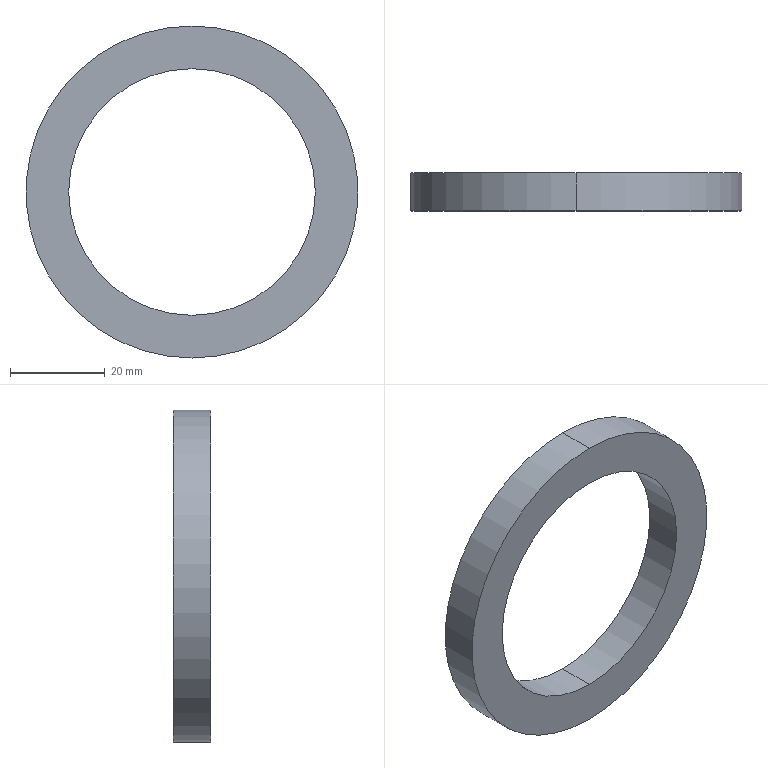Part | SolidWorks | features Extrusion 1 | 1 solid | 6 faces | box 70 x 8 x 70 mm | volume 13798 mm3 | cylinder 4 | plane 2 | commonest cylinder face diameters 52 x2 70 x2
STEP:
#1=CARTESIAN_POINT('',(0.,8.,-26.));
#2=VERTEX_POINT('',#1);
#3=CARTESIAN_POINT('',(0.,8.,26.));
#4=VERTEX_POINT('',#3);
#5=CARTESIAN_POINT('',(0.,8.,0.));
#6=DIRECTION('',(0.,1.,0.));
#7=DIRECTION('',(0.,0.,1.));
#8=AXIS2_PLACEMENT_3D('',#5,#6,#7);
#9=CIRCLE('',#8,26.);
#10=EDGE_CURVE('',#2,#4,#9,.T.);
#11=ORIENTED_EDGE('',*,*,#10,.T.);
#12=CARTESIAN_POINT('',(0.,0.,26.));
#13=VERTEX_POINT('',#12);
#14=CARTESIAN_POINT('',(0.,8.,26.));
#15=DIRECTION('',(0.,-1.,0.));
#16=VECTOR('',#15,1000.);
#17=LINE('',#14,#16);
#18=EDGE_CURVE('',#4,#13,#17,.T.);
#19=ORIENTED_EDGE('',*,*,#18,.T.);
#20=CARTESIAN_POINT('',(0.,0.,-26.));
#21=VERTEX_POINT('',#20);
#22=CARTESIAN_POINT('',(0.,0.,0.));
#23=DIRECTION('',(0.,1.,0.));
#24=DIRECTION('',(0.,0.,1.));
#25=AXIS2_PLACEMENT_3D('',#22,#23,#24);
#26=CIRCLE('',#25,26.);
#27=EDGE_CURVE('',#21,#13,#26,.T.);
#28=ORIENTED_EDGE('',*,*,#27,.F.);
#29=CARTESIAN_POINT('',(0.,8.,-26.));
#30=DIRECTION('',(0.,-1.,0.));
#31=VECTOR('',#30,1000.);
#32=LINE('',#29,#31);
#33=EDGE_CURVE('',#2,#21,#32,.T.);
#34=ORIENTED_EDGE('',*,*,#33,.F.);
#35=EDGE_LOOP('',(#11,#19,#28,#34));
#36=FACE_OUTER_BOUND('',#35,.T.);
#37=CARTESIAN_POINT('',(0.,8.,0.));
#38=DIRECTION('',(0.,-1.,0.));
#39=DIRECTION('',(0.,0.,-1.));
#40=AXIS2_PLACEMENT_3D('',#37,#38,#39);
#41=CYLINDRICAL_SURFACE('',#40,26.);
#42=ADVANCED_FACE('',(#36),#41,.F.);
#43=CARTESIAN_POINT('',(0.,8.,35.));
#44=VERTEX_POINT('',#43);
#45=CARTESIAN_POINT('',(0.,8.,-35.));
#46=VERTEX_POINT('',#45);
#47=CARTESIAN_POINT('',(0.,8.,0.));
#48=DIRECTION('',(0.,1.,0.));
#49=DIRECTION('',(0.,0.,1.));
#50=AXIS2_PLACEMENT_3D('',#47,#48,#49);
#51=CIRCLE('',#50,35.);
#52=EDGE_CURVE('',#44,#46,#51,.T.);
#53=ORIENTED_EDGE('',*,*,#52,.F.);
#54=CARTESIAN_POINT('',(0.,0.,35.));
#55=VERTEX_POINT('',#54);
#56=CARTESIAN_POINT('',(0.,8.,35.));
#57=DIRECTION('',(0.,-1.,0.));
#58=VECTOR('',#57,1000.);
#59=LINE('',#56,#58);
#60=EDGE_CURVE('',#44,#55,#59,.T.);
#61=ORIENTED_EDGE('',*,*,#60,.T.);
#62=CARTESIAN_POINT('',(0.,0.,-35.));
#63=VERTEX_POINT('',#62);
#64=CARTESIAN_POINT('',(0.,0.,0.));
#65=DIRECTION('',(0.,1.,0.));
#66=DIRECTION('',(0.,0.,1.));
#67=AXIS2_PLACEMENT_3D('',#64,#65,#66);
#68=CIRCLE('',#67,35.);
#69=EDGE_CURVE('',#55,#63,#68,.T.);
#70=ORIENTED_EDGE('',*,*,#69,.T.);
#71=CARTESIAN_POINT('',(0.,8.,-35.));
#72=DIRECTION('',(0.,-1.,0.));
#73=VECTOR('',#72,1000.);
#74=LINE('',#71,#73);
#75=EDGE_CURVE('',#46,#63,#74,.T.);
#76=ORIENTED_EDGE('',*,*,#75,.F.);
#77=EDGE_LOOP('',(#53,#61,#70,#76));
#78=FACE_OUTER_BOUND('',#77,.T.);
#79=CARTESIAN_POINT('',(0.,8.,0.));
#80=DIRECTION('',(0.,-1.,0.));
#81=DIRECTION('',(0.,0.,-1.));
#82=AXIS2_PLACEMENT_3D('',#79,#80,#81);
#83=CYLINDRICAL_SURFACE('',#82,35.);
#84=ADVANCED_FACE('',(#78),#83,.T.);
#85=CARTESIAN_POINT('',(0.,8.,0.));
#86=DIRECTION('',(0.,1.,0.));
#87=DIRECTION('',(0.,0.,1.));
#88=AXIS2_PLACEMENT_3D('',#85,#86,#87);
#89=CIRCLE('',#88,35.);
#90=EDGE_CURVE('',#46,#44,#89,.T.);
#91=ORIENTED_EDGE('',*,*,#90,.T.);
#92=ORIENTED_EDGE('',*,*,#52,.T.);
#93=EDGE_LOOP('',(#91,#92));
#94=FACE_OUTER_BOUND('',#93,.T.);
#95=ORIENTED_EDGE('',*,*,#10,.F.);
#96=CARTESIAN_POINT('',(0.,8.,0.));
#97=DIRECTION('',(0.,1.,0.));
#98=DIRECTION('',(0.,0.,1.));
#99=AXIS2_PLACEMENT_3D('',#96,#97,#98);
#100=CIRCLE('',#99,26.);
#101=EDGE_CURVE('',#4,#2,#100,.T.);
#102=ORIENTED_EDGE('',*,*,#101,.F.);
#103=EDGE_LOOP('',(#95,#102));
#104=FACE_BOUND('',#103,.T.);
#105=CARTESIAN_POINT('',(0.,8.,0.));
#106=DIRECTION('',(0.,1.,0.));
#107=DIRECTION('',(0.,0.,1.));
#108=AXIS2_PLACEMENT_3D('',#105,#106,#107);
#109=PLANE('',#108);
#110=ADVANCED_FACE('',(#94,#104),#109,.T.);
#111=CARTESIAN_POINT('',(0.,0.,0.));
#112=DIRECTION('',(0.,1.,0.));
#113=DIRECTION('',(0.,0.,1.));
#114=AXIS2_PLACEMENT_3D('',#111,#112,#113);
#115=CIRCLE('',#114,35.);
#116=EDGE_CURVE('',#63,#55,#115,.T.);
#117=ORIENTED_EDGE('',*,*,#116,.F.);
#118=ORIENTED_EDGE('',*,*,#69,.F.);
#119=EDGE_LOOP('',(#117,#118));
#120=FACE_OUTER_BOUND('',#119,.T.);
#121=ORIENTED_EDGE('',*,*,#27,.T.);
#122=CARTESIAN_POINT('',(0.,0.,0.));
#123=DIRECTION('',(0.,1.,0.));
#124=DIRECTION('',(0.,0.,1.));
#125=AXIS2_PLACEMENT_3D('',#122,#123,#124);
#126=CIRCLE('',#125,26.);
#127=EDGE_CURVE('',#13,#21,#126,.T.);
#128=ORIENTED_EDGE('',*,*,#127,.T.);
#129=EDGE_LOOP('',(#121,#128));
#130=FACE_BOUND('',#129,.T.);
#131=CARTESIAN_POINT('',(0.,0.,0.));
#132=DIRECTION('',(0.,1.,0.));
#133=DIRECTION('',(0.,0.,1.));
#134=AXIS2_PLACEMENT_3D('',#131,#132,#133);
#135=PLANE('',#134);
#136=ADVANCED_FACE('',(#120,#130),#135,.F.);
#137=ORIENTED_EDGE('',*,*,#60,.F.);
#138=ORIENTED_EDGE('',*,*,#90,.F.);
#139=ORIENTED_EDGE('',*,*,#75,.T.);
#140=ORIENTED_EDGE('',*,*,#116,.T.);
#141=EDGE_LOOP('',(#137,#138,#139,#140));
#142=FACE_OUTER_BOUND('',#141,.T.);
#143=CARTESIAN_POINT('',(0.,8.,0.));
#144=DIRECTION('',(0.,-1.,0.));
#145=DIRECTION('',(0.,0.,-1.));
#146=AXIS2_PLACEMENT_3D('',#143,#144,#145);
#147=CYLINDRICAL_SURFACE('',#146,35.);
#148=ADVANCED_FACE('',(#142),#147,.T.);
#149=ORIENTED_EDGE('',*,*,#18,.F.);
#150=ORIENTED_EDGE('',*,*,#101,.T.);
#151=ORIENTED_EDGE('',*,*,#33,.T.);
#152=ORIENTED_EDGE('',*,*,#127,.F.);
#153=EDGE_LOOP('',(#149,#150,#151,#152));
#154=FACE_OUTER_BOUND('',#153,.T.);
#155=CARTESIAN_POINT('',(0.,8.,0.));
#156=DIRECTION('',(0.,-1.,0.));
#157=DIRECTION('',(0.,0.,-1.));
#158=AXIS2_PLACEMENT_3D('',#155,#156,#157);
#159=CYLINDRICAL_SURFACE('',#158,26.);
#160=ADVANCED_FACE('',(#154),#159,.F.);
#161=CLOSED_SHELL('',(#42,#84,#110,#136,#148,#160));
#162=MANIFOLD_SOLID_BREP('',#161);
#163=CARTESIAN_POINT('',(0.,0.,0.));
#164=DIRECTION('',(0.,0.,1.));
#165=DIRECTION('',(1.,0.,0.));
#166=AXIS2_PLACEMENT_3D('',#163,#164,#165);
#167=(LENGTH_UNIT()NAMED_UNIT(*)SI_UNIT(.MILLI.,.METRE.));
#168=UNCERTAINTY_MEASURE_WITH_UNIT(LENGTH_MEASURE(0.00001),#167,'','');
#169=(NAMED_UNIT(*)PLANE_ANGLE_UNIT()SI_UNIT($,.RADIAN.));
#170=(NAMED_UNIT(*)SI_UNIT($,.STERADIAN.)SOLID_ANGLE_UNIT());
#171=(GEOMETRIC_REPRESENTATION_CONTEXT(3)GLOBAL_UNCERTAINTY_ASSIGNED_CONTEXT((#168))GLOBAL_UNIT_ASSIGNED_CONTEXT((#167,#169,#170))REPRESENTATION_CONTEXT('',''));
#172=ADVANCED_BREP_SHAPE_REPRESENTATION('',(#162,#166),#171);